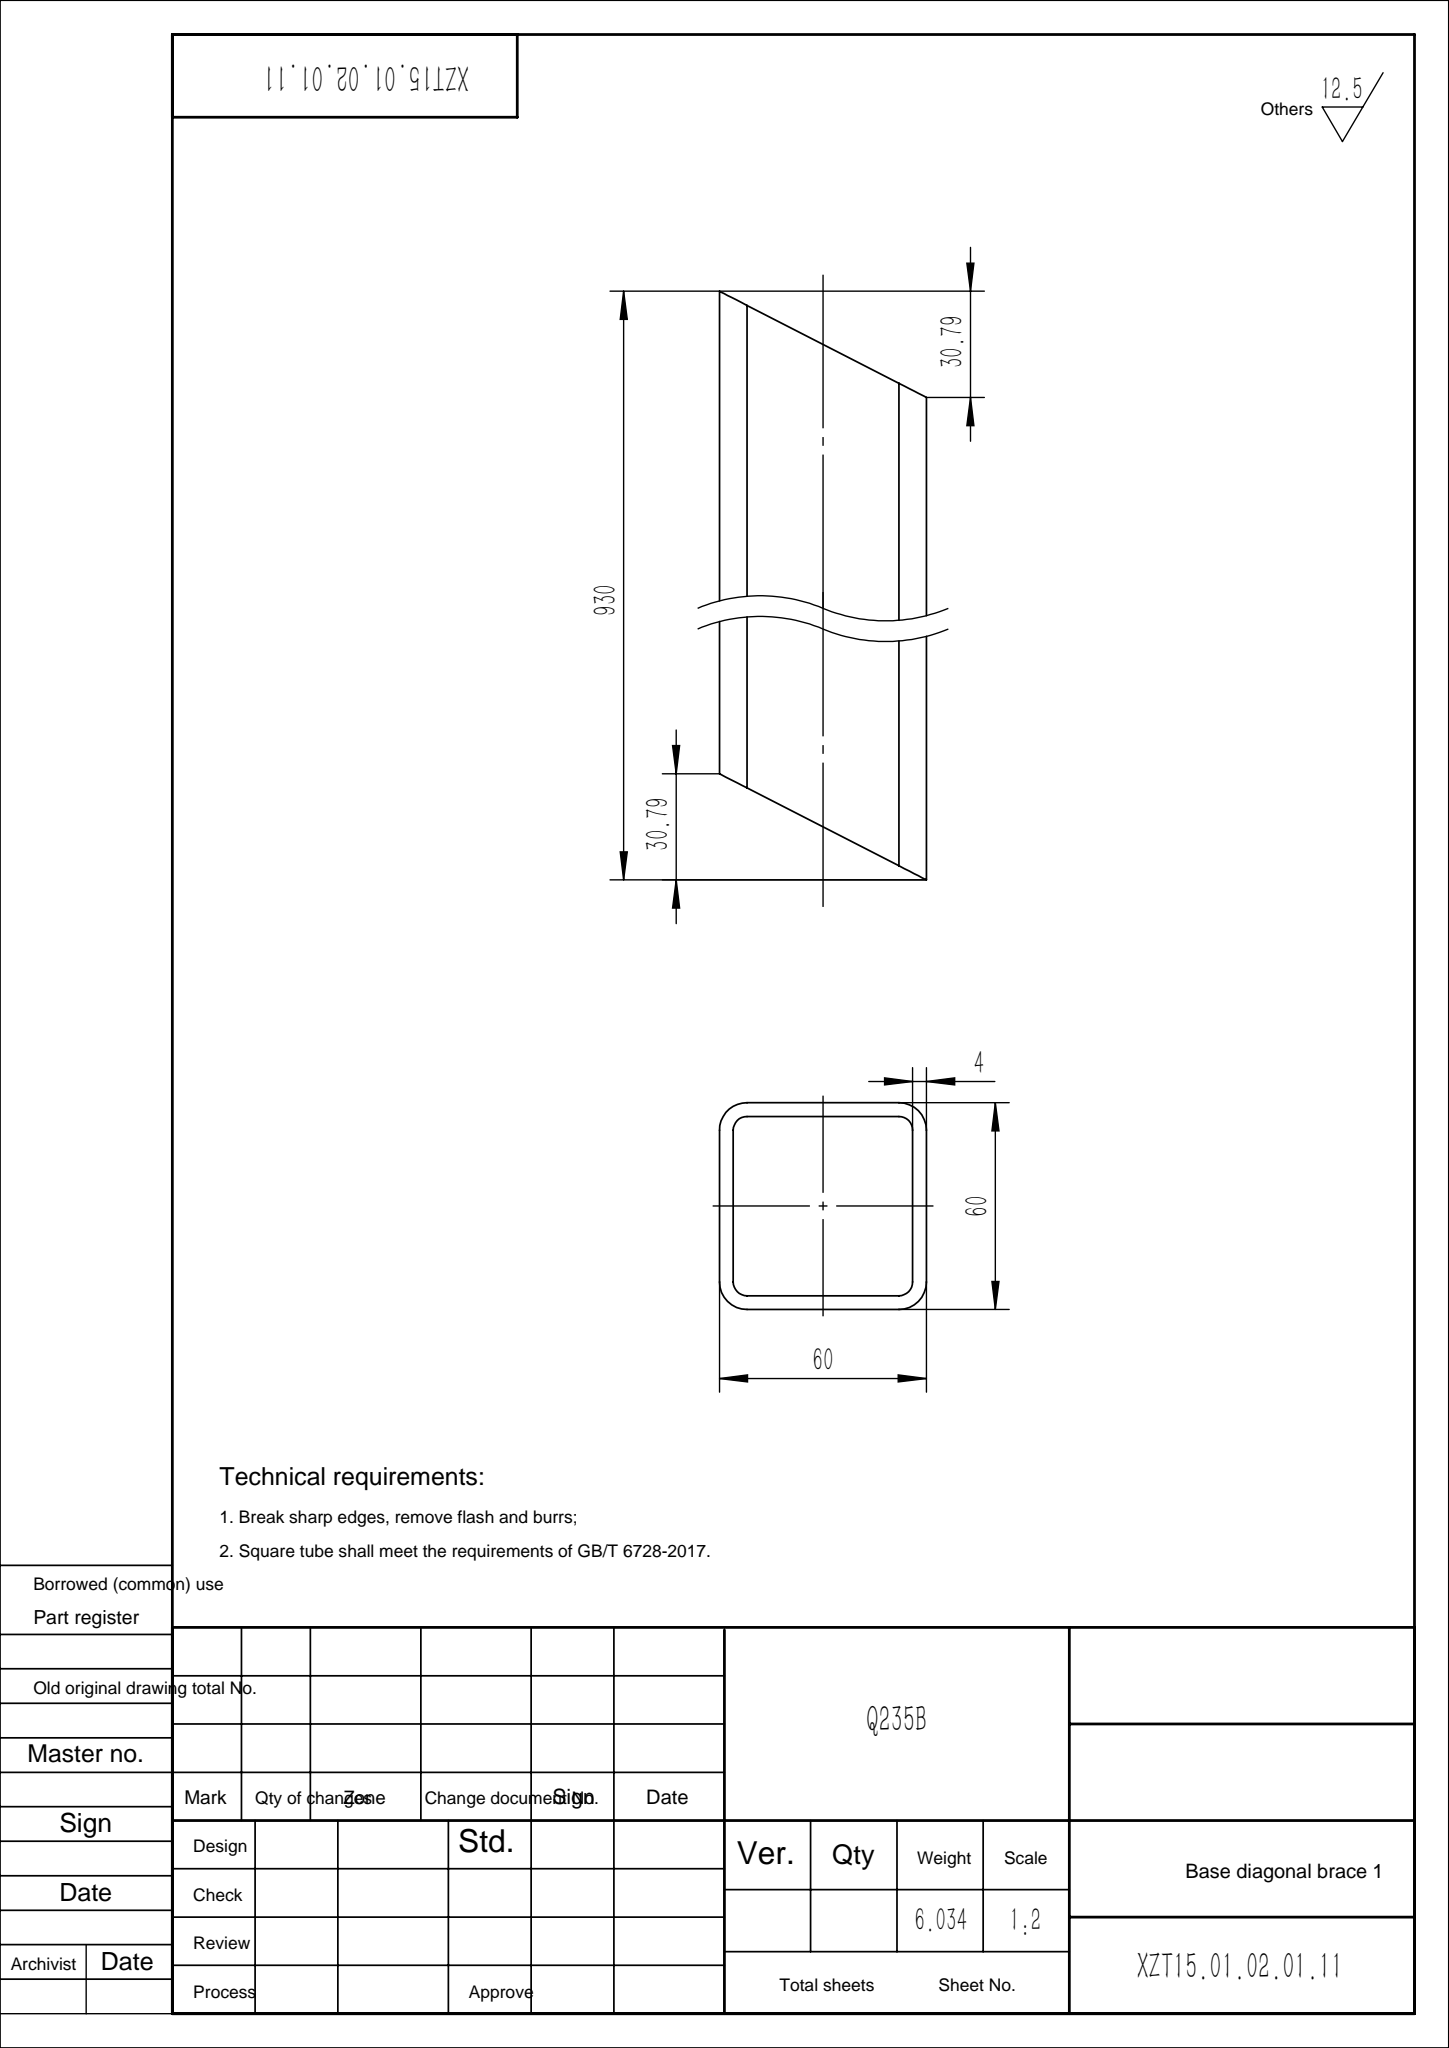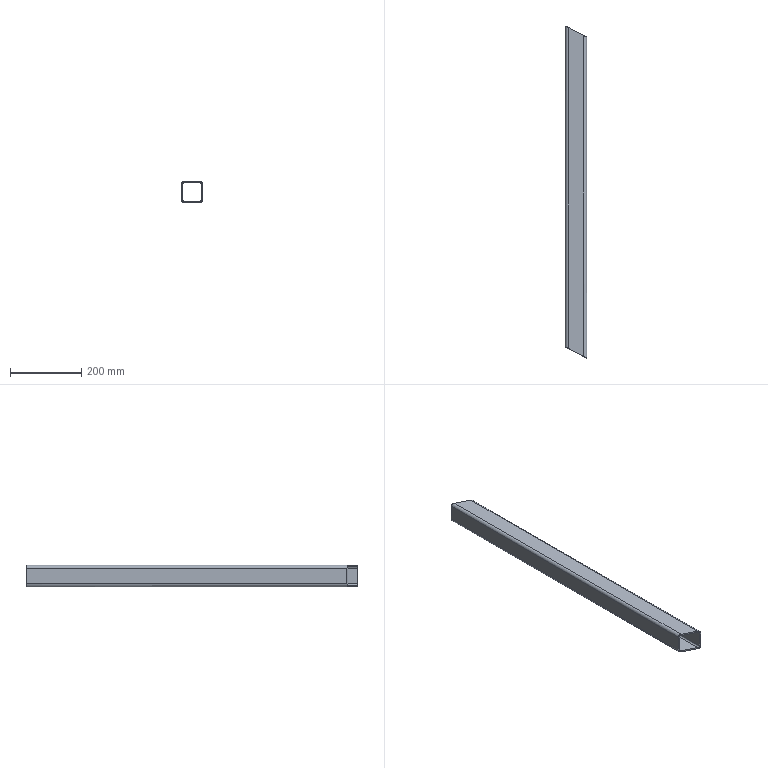Part | SolidWorks | features ICE 1, WeldMemberFeat 1, WeldmentFeature 1 | 1 solid | 18 faces | box 60 x 930 x 60 mm | volume 768639 mm3 | plane 10 | cylinder 8 | commonest cylinder face diameters 8 x4 16 x4
STEP:
#1=CARTESIAN_POINT('',(30.,899.207,-22.));
#2=VERTEX_POINT('',#1);
#3=CARTESIAN_POINT('',(30.,0.,-22.));
#4=VERTEX_POINT('',#3);
#5=CARTESIAN_POINT('',(30.,930.,-22.));
#6=DIRECTION('',(0.,-1.,0.));
#7=VECTOR('',#6,1000.);
#8=LINE('',#5,#7);
#9=EDGE_CURVE('',#2,#4,#8,.T.);
#10=ORIENTED_EDGE('',*,*,#9,.F.);
#11=CARTESIAN_POINT('',(30.,899.207,22.));
#12=VERTEX_POINT('',#11);
#13=CARTESIAN_POINT('',(30.,899.207,-30.));
#14=DIRECTION('',(0.,0.,1.));
#15=VECTOR('',#14,1000.);
#16=LINE('',#13,#15);
#17=EDGE_CURVE('',#2,#12,#16,.T.);
#18=ORIENTED_EDGE('',*,*,#17,.T.);
#19=CARTESIAN_POINT('',(30.,0.,22.));
#20=VERTEX_POINT('',#19);
#21=CARTESIAN_POINT('',(30.,930.,22.));
#22=DIRECTION('',(0.,-1.,0.));
#23=VECTOR('',#22,1000.);
#24=LINE('',#21,#23);
#25=EDGE_CURVE('',#12,#20,#24,.T.);
#26=ORIENTED_EDGE('',*,*,#25,.T.);
#27=CARTESIAN_POINT('',(30.,0.,-22.));
#28=DIRECTION('',(0.,0.,-1.));
#29=VECTOR('',#28,1000.);
#30=LINE('',#27,#29);
#31=EDGE_CURVE('',#20,#4,#30,.T.);
#32=ORIENTED_EDGE('',*,*,#31,.T.);
#33=EDGE_LOOP('',(#10,#18,#26,#32));
#34=FACE_OUTER_BOUND('',#33,.T.);
#35=CARTESIAN_POINT('',(30.,930.,-22.));
#36=DIRECTION('',(-1.,0.,0.));
#37=DIRECTION('',(0.,0.,1.));
#38=AXIS2_PLACEMENT_3D('',#35,#36,#37);
#39=PLANE('',#38);
#40=ADVANCED_FACE('',(#34),#39,.F.);
#41=CARTESIAN_POINT('',(-30.,930.,-22.));
#42=VERTEX_POINT('',#41);
#43=CARTESIAN_POINT('',(-30.,30.793,-22.));
#44=VERTEX_POINT('',#43);
#45=CARTESIAN_POINT('',(-30.,930.,-22.));
#46=DIRECTION('',(0.,-1.,0.));
#47=VECTOR('',#46,1000.);
#48=LINE('',#45,#47);
#49=EDGE_CURVE('',#42,#44,#48,.T.);
#50=ORIENTED_EDGE('',*,*,#49,.T.);
#51=CARTESIAN_POINT('',(-30.,30.793,22.));
#52=VERTEX_POINT('',#51);
#53=CARTESIAN_POINT('',(-30.,30.793,-30.));
#54=DIRECTION('',(0.,0.,1.));
#55=VECTOR('',#54,1000.);
#56=LINE('',#53,#55);
#57=EDGE_CURVE('',#44,#52,#56,.T.);
#58=ORIENTED_EDGE('',*,*,#57,.T.);
#59=CARTESIAN_POINT('',(-30.,930.,22.));
#60=VERTEX_POINT('',#59);
#61=CARTESIAN_POINT('',(-30.,930.,22.));
#62=DIRECTION('',(0.,-1.,0.));
#63=VECTOR('',#62,1000.);
#64=LINE('',#61,#63);
#65=EDGE_CURVE('',#60,#52,#64,.T.);
#66=ORIENTED_EDGE('',*,*,#65,.F.);
#67=CARTESIAN_POINT('',(-30.,930.,22.));
#68=DIRECTION('',(0.,0.,1.));
#69=VECTOR('',#68,1000.);
#70=LINE('',#67,#69);
#71=EDGE_CURVE('',#42,#60,#70,.T.);
#72=ORIENTED_EDGE('',*,*,#71,.F.);
#73=EDGE_LOOP('',(#50,#58,#66,#72));
#74=FACE_OUTER_BOUND('',#73,.T.);
#75=CARTESIAN_POINT('',(-30.,930.,22.));
#76=DIRECTION('',(1.,0.,0.));
#77=DIRECTION('',(0.,0.,-1.));
#78=AXIS2_PLACEMENT_3D('',#75,#76,#77);
#79=PLANE('',#78);
#80=ADVANCED_FACE('',(#74),#79,.F.);
#81=ORIENTED_EDGE('',*,*,#49,.F.);
#82=CARTESIAN_POINT('',(-22.,925.894,-30.));
#83=VERTEX_POINT('',#82);
#84=CARTESIAN_POINT('',(-30.,930.,-22.));
#85=CARTESIAN_POINT('',(-30.,930.,-26.686));
#86=CARTESIAN_POINT('',(-26.686,928.299,-30.));
#87=CARTESIAN_POINT('',(-22.,925.894,-30.));
#88=(BOUNDED_CURVE()B_SPLINE_CURVE(3,(#84,#85,#86,#87),.UNSPECIFIED.,.F.,.T.)B_SPLINE_CURVE_WITH_KNOTS((4,4),(3.142,4.712),.UNSPECIFIED.)CURVE()GEOMETRIC_REPRESENTATION_ITEM()RATIONAL_B_SPLINE_CURVE((1.,0.8047,0.8047,1.))REPRESENTATION_ITEM(''));
#89=EDGE_CURVE('',#42,#83,#88,.T.);
#90=ORIENTED_EDGE('',*,*,#89,.T.);
#91=CARTESIAN_POINT('',(-22.,26.687,-30.));
#92=VERTEX_POINT('',#91);
#93=CARTESIAN_POINT('',(-22.,930.,-30.));
#94=DIRECTION('',(0.,-1.,0.));
#95=VECTOR('',#94,1000.);
#96=LINE('',#93,#95);
#97=EDGE_CURVE('',#83,#92,#96,.T.);
#98=ORIENTED_EDGE('',*,*,#97,.T.);
#99=CARTESIAN_POINT('',(-22.,26.687,-30.));
#100=CARTESIAN_POINT('',(-26.686,29.093,-30.));
#101=CARTESIAN_POINT('',(-30.,30.793,-26.686));
#102=CARTESIAN_POINT('',(-30.,30.793,-22.));
#103=(BOUNDED_CURVE()B_SPLINE_CURVE(3,(#99,#100,#101,#102),.UNSPECIFIED.,.F.,.T.)B_SPLINE_CURVE_WITH_KNOTS((4,4),(1.571,3.142),.UNSPECIFIED.)CURVE()GEOMETRIC_REPRESENTATION_ITEM()RATIONAL_B_SPLINE_CURVE((1.,0.8047,0.8047,1.))REPRESENTATION_ITEM(''));
#104=EDGE_CURVE('',#92,#44,#103,.T.);
#105=ORIENTED_EDGE('',*,*,#104,.T.);
#106=EDGE_LOOP('',(#81,#90,#98,#105));
#107=FACE_OUTER_BOUND('',#106,.T.);
#108=CARTESIAN_POINT('',(-22.,930.,-22.));
#109=DIRECTION('',(0.,-1.,0.));
#110=DIRECTION('',(0.,0.,-1.));
#111=AXIS2_PLACEMENT_3D('',#108,#109,#110);
#112=CYLINDRICAL_SURFACE('',#111,8.);
#113=ADVANCED_FACE('',(#107),#112,.T.);
#114=ORIENTED_EDGE('',*,*,#97,.F.);
#115=CARTESIAN_POINT('',(22.,903.313,-30.));
#116=VERTEX_POINT('',#115);
#117=CARTESIAN_POINT('',(-30.,930.,-30.));
#118=DIRECTION('',(0.8897,-0.4566,0.));
#119=VECTOR('',#118,1000.);
#120=LINE('',#117,#119);
#121=EDGE_CURVE('',#83,#116,#120,.T.);
#122=ORIENTED_EDGE('',*,*,#121,.T.);
#123=CARTESIAN_POINT('',(22.,4.106,-30.));
#124=VERTEX_POINT('',#123);
#125=CARTESIAN_POINT('',(22.,930.,-30.));
#126=DIRECTION('',(0.,-1.,0.));
#127=VECTOR('',#126,1000.);
#128=LINE('',#125,#127);
#129=EDGE_CURVE('',#116,#124,#128,.T.);
#130=ORIENTED_EDGE('',*,*,#129,.T.);
#131=CARTESIAN_POINT('',(-30.,30.793,-30.));
#132=DIRECTION('',(-0.8897,0.4566,0.));
#133=VECTOR('',#132,1000.);
#134=LINE('',#131,#133);
#135=EDGE_CURVE('',#124,#92,#134,.T.);
#136=ORIENTED_EDGE('',*,*,#135,.T.);
#137=EDGE_LOOP('',(#114,#122,#130,#136));
#138=FACE_OUTER_BOUND('',#137,.T.);
#139=CARTESIAN_POINT('',(22.,930.,-30.));
#140=DIRECTION('',(0.,0.,1.));
#141=DIRECTION('',(1.,0.,0.));
#142=AXIS2_PLACEMENT_3D('',#139,#140,#141);
#143=PLANE('',#142);
#144=ADVANCED_FACE('',(#138),#143,.F.);
#145=ORIENTED_EDGE('',*,*,#129,.F.);
#146=CARTESIAN_POINT('',(22.,903.313,-30.));
#147=CARTESIAN_POINT('',(26.686,900.907,-30.));
#148=CARTESIAN_POINT('',(30.,899.207,-26.686));
#149=CARTESIAN_POINT('',(30.,899.207,-22.));
#150=(BOUNDED_CURVE()B_SPLINE_CURVE(3,(#146,#147,#148,#149),.UNSPECIFIED.,.F.,.F.)B_SPLINE_CURVE_WITH_KNOTS((4,4),(4.712,6.283),.UNSPECIFIED.)CURVE()GEOMETRIC_REPRESENTATION_ITEM()RATIONAL_B_SPLINE_CURVE((1.,0.8047,0.8047,1.))REPRESENTATION_ITEM(''));
#151=EDGE_CURVE('',#116,#2,#150,.T.);
#152=ORIENTED_EDGE('',*,*,#151,.T.);
#153=ORIENTED_EDGE('',*,*,#9,.T.);
#154=CARTESIAN_POINT('',(30.,0.,-22.));
#155=CARTESIAN_POINT('',(30.,0.,-26.686));
#156=CARTESIAN_POINT('',(26.686,1.701,-30.));
#157=CARTESIAN_POINT('',(22.,4.106,-30.));
#158=(BOUNDED_CURVE()B_SPLINE_CURVE(3,(#154,#155,#156,#157),.UNSPECIFIED.,.F.,.T.)B_SPLINE_CURVE_WITH_KNOTS((4,4),(0.,1.571),.UNSPECIFIED.)CURVE()GEOMETRIC_REPRESENTATION_ITEM()RATIONAL_B_SPLINE_CURVE((1.,0.8047,0.8047,1.))REPRESENTATION_ITEM(''));
#159=EDGE_CURVE('',#4,#124,#158,.T.);
#160=ORIENTED_EDGE('',*,*,#159,.T.);
#161=EDGE_LOOP('',(#145,#152,#153,#160));
#162=FACE_OUTER_BOUND('',#161,.T.);
#163=CARTESIAN_POINT('',(22.,930.,-22.));
#164=DIRECTION('',(0.,-1.,0.));
#165=DIRECTION('',(0.,0.,-1.));
#166=AXIS2_PLACEMENT_3D('',#163,#164,#165);
#167=CYLINDRICAL_SURFACE('',#166,8.);
#168=ADVANCED_FACE('',(#162),#167,.T.);
#169=ORIENTED_EDGE('',*,*,#25,.F.);
#170=CARTESIAN_POINT('',(22.,903.313,30.));
#171=VERTEX_POINT('',#170);
#172=CARTESIAN_POINT('',(30.,899.207,22.));
#173=CARTESIAN_POINT('',(30.,899.207,26.686));
#174=CARTESIAN_POINT('',(26.686,900.907,30.));
#175=CARTESIAN_POINT('',(22.,903.313,30.));
#176=(BOUNDED_CURVE()B_SPLINE_CURVE(3,(#172,#173,#174,#175),.UNSPECIFIED.,.F.,.T.)B_SPLINE_CURVE_WITH_KNOTS((4,4),(0.,1.571),.UNSPECIFIED.)CURVE()GEOMETRIC_REPRESENTATION_ITEM()RATIONAL_B_SPLINE_CURVE((1.,0.8047,0.8047,1.))REPRESENTATION_ITEM(''));
#177=EDGE_CURVE('',#12,#171,#176,.T.);
#178=ORIENTED_EDGE('',*,*,#177,.T.);
#179=CARTESIAN_POINT('',(22.,4.106,30.));
#180=VERTEX_POINT('',#179);
#181=CARTESIAN_POINT('',(22.,930.,30.));
#182=DIRECTION('',(0.,-1.,0.));
#183=VECTOR('',#182,1000.);
#184=LINE('',#181,#183);
#185=EDGE_CURVE('',#171,#180,#184,.T.);
#186=ORIENTED_EDGE('',*,*,#185,.T.);
#187=CARTESIAN_POINT('',(22.,4.106,30.));
#188=CARTESIAN_POINT('',(26.686,1.701,30.));
#189=CARTESIAN_POINT('',(30.,0.,26.686));
#190=CARTESIAN_POINT('',(30.,0.,22.));
#191=(BOUNDED_CURVE()B_SPLINE_CURVE(3,(#187,#188,#189,#190),.UNSPECIFIED.,.F.,.T.)B_SPLINE_CURVE_WITH_KNOTS((4,4),(4.712,6.283),.UNSPECIFIED.)CURVE()GEOMETRIC_REPRESENTATION_ITEM()RATIONAL_B_SPLINE_CURVE((1.,0.8047,0.8047,1.))REPRESENTATION_ITEM(''));
#192=EDGE_CURVE('',#180,#20,#191,.T.);
#193=ORIENTED_EDGE('',*,*,#192,.T.);
#194=EDGE_LOOP('',(#169,#178,#186,#193));
#195=FACE_OUTER_BOUND('',#194,.T.);
#196=CARTESIAN_POINT('',(22.,930.,22.));
#197=DIRECTION('',(0.,-1.,0.));
#198=DIRECTION('',(0.,0.,-1.));
#199=AXIS2_PLACEMENT_3D('',#196,#197,#198);
#200=CYLINDRICAL_SURFACE('',#199,8.);
#201=ADVANCED_FACE('',(#195),#200,.T.);
#202=ORIENTED_EDGE('',*,*,#185,.F.);
#203=CARTESIAN_POINT('',(-22.,925.894,30.));
#204=VERTEX_POINT('',#203);
#205=CARTESIAN_POINT('',(-23.668,926.75,30.));
#206=DIRECTION('',(-0.8897,0.4566,0.));
#207=VECTOR('',#206,1000.);
#208=LINE('',#205,#207);
#209=EDGE_CURVE('',#171,#204,#208,.T.);
#210=ORIENTED_EDGE('',*,*,#209,.T.);
#211=CARTESIAN_POINT('',(-22.,26.687,30.));
#212=VERTEX_POINT('',#211);
#213=CARTESIAN_POINT('',(-22.,930.,30.));
#214=DIRECTION('',(0.,-1.,0.));
#215=VECTOR('',#214,1000.);
#216=LINE('',#213,#215);
#217=EDGE_CURVE('',#204,#212,#216,.T.);
#218=ORIENTED_EDGE('',*,*,#217,.T.);
#219=CARTESIAN_POINT('',(-388.946,215.012,30.));
#220=DIRECTION('',(0.8897,-0.4566,0.));
#221=VECTOR('',#220,1000.);
#222=LINE('',#219,#221);
#223=EDGE_CURVE('',#212,#180,#222,.T.);
#224=ORIENTED_EDGE('',*,*,#223,.T.);
#225=EDGE_LOOP('',(#202,#210,#218,#224));
#226=FACE_OUTER_BOUND('',#225,.T.);
#227=CARTESIAN_POINT('',(-22.,930.,30.));
#228=DIRECTION('',(0.,0.,-1.));
#229=DIRECTION('',(-1.,0.,0.));
#230=AXIS2_PLACEMENT_3D('',#227,#228,#229);
#231=PLANE('',#230);
#232=ADVANCED_FACE('',(#226),#231,.F.);
#233=ORIENTED_EDGE('',*,*,#217,.F.);
#234=CARTESIAN_POINT('',(-22.,925.894,30.));
#235=CARTESIAN_POINT('',(-26.686,928.299,30.));
#236=CARTESIAN_POINT('',(-30.,930.,26.686));
#237=CARTESIAN_POINT('',(-30.,930.,22.));
#238=(BOUNDED_CURVE()B_SPLINE_CURVE(3,(#234,#235,#236,#237),.UNSPECIFIED.,.F.,.T.)B_SPLINE_CURVE_WITH_KNOTS((4,4),(1.571,3.142),.UNSPECIFIED.)CURVE()GEOMETRIC_REPRESENTATION_ITEM()RATIONAL_B_SPLINE_CURVE((1.,0.8047,0.8047,1.))REPRESENTATION_ITEM(''));
#239=EDGE_CURVE('',#204,#60,#238,.T.);
#240=ORIENTED_EDGE('',*,*,#239,.T.);
#241=ORIENTED_EDGE('',*,*,#65,.T.);
#242=CARTESIAN_POINT('',(-30.,30.793,22.));
#243=CARTESIAN_POINT('',(-30.,30.793,26.686));
#244=CARTESIAN_POINT('',(-26.686,29.093,30.));
#245=CARTESIAN_POINT('',(-22.,26.687,30.));
#246=(BOUNDED_CURVE()B_SPLINE_CURVE(3,(#242,#243,#244,#245),.UNSPECIFIED.,.F.,.F.)B_SPLINE_CURVE_WITH_KNOTS((4,4),(3.142,4.712),.UNSPECIFIED.)CURVE()GEOMETRIC_REPRESENTATION_ITEM()RATIONAL_B_SPLINE_CURVE((1.,0.8047,0.8047,1.))REPRESENTATION_ITEM(''));
#247=EDGE_CURVE('',#52,#212,#246,.T.);
#248=ORIENTED_EDGE('',*,*,#247,.T.);
#249=EDGE_LOOP('',(#233,#240,#241,#248));
#250=FACE_OUTER_BOUND('',#249,.T.);
#251=CARTESIAN_POINT('',(-22.,930.,22.));
#252=DIRECTION('',(0.,-1.,0.));
#253=DIRECTION('',(0.,0.,-1.));
#254=AXIS2_PLACEMENT_3D('',#251,#252,#253);
#255=CYLINDRICAL_SURFACE('',#254,8.);
#256=ADVANCED_FACE('',(#250),#255,.T.);
#257=CARTESIAN_POINT('',(22.,4.106,26.));
#258=VERTEX_POINT('',#257);
#259=CARTESIAN_POINT('',(26.,2.053,22.));
#260=VERTEX_POINT('',#259);
#261=CARTESIAN_POINT('',(22.,4.106,26.));
#262=CARTESIAN_POINT('',(24.343,2.903,26.));
#263=CARTESIAN_POINT('',(26.,2.053,24.343));
#264=CARTESIAN_POINT('',(26.,2.053,22.));
#265=(BOUNDED_CURVE()B_SPLINE_CURVE(3,(#261,#262,#263,#264),.UNSPECIFIED.,.F.,.T.)B_SPLINE_CURVE_WITH_KNOTS((4,4),(4.712,6.283),.UNSPECIFIED.)CURVE()GEOMETRIC_REPRESENTATION_ITEM()RATIONAL_B_SPLINE_CURVE((1.,0.8047,0.8047,1.))REPRESENTATION_ITEM(''));
#266=EDGE_CURVE('',#258,#260,#265,.T.);
#267=ORIENTED_EDGE('',*,*,#266,.T.);
#268=CARTESIAN_POINT('',(26.,2.053,-22.));
#269=VERTEX_POINT('',#268);
#270=CARTESIAN_POINT('',(26.,2.053,-22.));
#271=DIRECTION('',(0.,0.,-1.));
#272=VECTOR('',#271,1000.);
#273=LINE('',#270,#272);
#274=EDGE_CURVE('',#260,#269,#273,.T.);
#275=ORIENTED_EDGE('',*,*,#274,.T.);
#276=CARTESIAN_POINT('',(22.,4.106,-26.));
#277=VERTEX_POINT('',#276);
#278=CARTESIAN_POINT('',(26.,2.053,-22.));
#279=CARTESIAN_POINT('',(26.,2.053,-24.343));
#280=CARTESIAN_POINT('',(24.343,2.903,-26.));
#281=CARTESIAN_POINT('',(22.,4.106,-26.));
#282=(BOUNDED_CURVE()B_SPLINE_CURVE(3,(#278,#279,#280,#281),.UNSPECIFIED.,.F.,.T.)B_SPLINE_CURVE_WITH_KNOTS((4,4),(0.,1.571),.UNSPECIFIED.)CURVE()GEOMETRIC_REPRESENTATION_ITEM()RATIONAL_B_SPLINE_CURVE((1.,0.8047,0.8047,1.))REPRESENTATION_ITEM(''));
#283=EDGE_CURVE('',#269,#277,#282,.T.);
#284=ORIENTED_EDGE('',*,*,#283,.T.);
#285=CARTESIAN_POINT('',(-22.,26.687,-26.));
#286=VERTEX_POINT('',#285);
#287=CARTESIAN_POINT('',(-354.12,197.138,-26.));
#288=DIRECTION('',(-0.8897,0.4566,0.));
#289=VECTOR('',#288,1000.);
#290=LINE('',#287,#289);
#291=EDGE_CURVE('',#277,#286,#290,.T.);
#292=ORIENTED_EDGE('',*,*,#291,.T.);
#293=CARTESIAN_POINT('',(-26.,28.74,-22.));
#294=VERTEX_POINT('',#293);
#295=CARTESIAN_POINT('',(-22.,26.687,-26.));
#296=CARTESIAN_POINT('',(-24.343,27.89,-26.));
#297=CARTESIAN_POINT('',(-26.,28.74,-24.343));
#298=CARTESIAN_POINT('',(-26.,28.74,-22.));
#299=(BOUNDED_CURVE()B_SPLINE_CURVE(3,(#295,#296,#297,#298),.UNSPECIFIED.,.F.,.T.)B_SPLINE_CURVE_WITH_KNOTS((4,4),(1.571,3.142),.UNSPECIFIED.)CURVE()GEOMETRIC_REPRESENTATION_ITEM()RATIONAL_B_SPLINE_CURVE((1.,0.8047,0.8047,1.))REPRESENTATION_ITEM(''));
#300=EDGE_CURVE('',#286,#294,#299,.T.);
#301=ORIENTED_EDGE('',*,*,#300,.T.);
#302=CARTESIAN_POINT('',(-26.,28.74,22.));
#303=VERTEX_POINT('',#302);
#304=CARTESIAN_POINT('',(-26.,28.74,22.));
#305=DIRECTION('',(0.,0.,1.));
#306=VECTOR('',#305,1000.);
#307=LINE('',#304,#306);
#308=EDGE_CURVE('',#294,#303,#307,.T.);
#309=ORIENTED_EDGE('',*,*,#308,.T.);
#310=CARTESIAN_POINT('',(-22.,26.687,26.));
#311=VERTEX_POINT('',#310);
#312=CARTESIAN_POINT('',(-26.,28.74,22.));
#313=CARTESIAN_POINT('',(-26.,28.74,24.343));
#314=CARTESIAN_POINT('',(-24.343,27.89,26.));
#315=CARTESIAN_POINT('',(-22.,26.687,26.));
#316=(BOUNDED_CURVE()B_SPLINE_CURVE(3,(#312,#313,#314,#315),.UNSPECIFIED.,.F.,.F.)B_SPLINE_CURVE_WITH_KNOTS((4,4),(3.142,4.712),.UNSPECIFIED.)CURVE()GEOMETRIC_REPRESENTATION_ITEM()RATIONAL_B_SPLINE_CURVE((1.,0.8047,0.8047,1.))REPRESENTATION_ITEM(''));
#317=EDGE_CURVE('',#303,#311,#316,.T.);
#318=ORIENTED_EDGE('',*,*,#317,.T.);
#319=CARTESIAN_POINT('',(-388.946,215.012,26.));
#320=DIRECTION('',(0.8897,-0.4566,0.));
#321=VECTOR('',#320,1000.);
#322=LINE('',#319,#321);
#323=EDGE_CURVE('',#311,#258,#322,.T.);
#324=ORIENTED_EDGE('',*,*,#323,.T.);
#325=EDGE_LOOP('',(#267,#275,#284,#292,#301,#309,#318,#324));
#326=FACE_BOUND('',#325,.T.);
#327=ORIENTED_EDGE('',*,*,#57,.F.);
#328=ORIENTED_EDGE('',*,*,#104,.F.);
#329=ORIENTED_EDGE('',*,*,#135,.F.);
#330=ORIENTED_EDGE('',*,*,#159,.F.);
#331=ORIENTED_EDGE('',*,*,#31,.F.);
#332=ORIENTED_EDGE('',*,*,#192,.F.);
#333=ORIENTED_EDGE('',*,*,#223,.F.);
#334=ORIENTED_EDGE('',*,*,#247,.F.);
#335=EDGE_LOOP('',(#327,#328,#329,#330,#331,#332,#333,#334));
#336=FACE_OUTER_BOUND('',#335,.T.);
#337=CARTESIAN_POINT('',(-30.,30.793,-30.));
#338=DIRECTION('',(0.4566,0.8897,0.));
#339=DIRECTION('',(-0.8897,0.4566,0.));
#340=AXIS2_PLACEMENT_3D('',#337,#338,#339);
#341=PLANE('',#340);
#342=ADVANCED_FACE('',(#326,#336),#341,.F.);
#343=CARTESIAN_POINT('',(26.,901.26,22.));
#344=VERTEX_POINT('',#343);
#345=CARTESIAN_POINT('',(22.,903.313,26.));
#346=VERTEX_POINT('',#345);
#347=CARTESIAN_POINT('',(26.,901.26,22.));
#348=CARTESIAN_POINT('',(26.,901.26,24.343));
#349=CARTESIAN_POINT('',(24.343,902.11,26.));
#350=CARTESIAN_POINT('',(22.,903.313,26.));
#351=(BOUNDED_CURVE()B_SPLINE_CURVE(3,(#347,#348,#349,#350),.UNSPECIFIED.,.F.,.T.)B_SPLINE_CURVE_WITH_KNOTS((4,4),(0.,1.571),.UNSPECIFIED.)CURVE()GEOMETRIC_REPRESENTATION_ITEM()RATIONAL_B_SPLINE_CURVE((1.,0.8047,0.8047,1.))REPRESENTATION_ITEM(''));
#352=EDGE_CURVE('',#344,#346,#351,.T.);
#353=ORIENTED_EDGE('',*,*,#352,.T.);
#354=CARTESIAN_POINT('',(-22.,925.894,26.));
#355=VERTEX_POINT('',#354);
#356=CARTESIAN_POINT('',(-23.668,926.75,26.));
#357=DIRECTION('',(-0.8897,0.4566,0.));
#358=VECTOR('',#357,1000.);
#359=LINE('',#356,#358);
#360=EDGE_CURVE('',#346,#355,#359,.T.);
#361=ORIENTED_EDGE('',*,*,#360,.T.);
#362=CARTESIAN_POINT('',(-26.,927.947,22.));
#363=VERTEX_POINT('',#362);
#364=CARTESIAN_POINT('',(-22.,925.894,26.));
#365=CARTESIAN_POINT('',(-24.343,927.097,26.));
#366=CARTESIAN_POINT('',(-26.,927.947,24.343));
#367=CARTESIAN_POINT('',(-26.,927.947,22.));
#368=(BOUNDED_CURVE()B_SPLINE_CURVE(3,(#364,#365,#366,#367),.UNSPECIFIED.,.F.,.F.)B_SPLINE_CURVE_WITH_KNOTS((4,4),(1.571,3.142),.UNSPECIFIED.)CURVE()GEOMETRIC_REPRESENTATION_ITEM()RATIONAL_B_SPLINE_CURVE((1.,0.8047,0.8047,1.))REPRESENTATION_ITEM(''));
#369=EDGE_CURVE('',#355,#363,#368,.T.);
#370=ORIENTED_EDGE('',*,*,#369,.T.);
#371=CARTESIAN_POINT('',(-26.,927.947,-22.));
#372=VERTEX_POINT('',#371);
#373=CARTESIAN_POINT('',(-26.,927.947,22.));
#374=DIRECTION('',(0.,0.,-1.));
#375=VECTOR('',#374,1000.);
#376=LINE('',#373,#375);
#377=EDGE_CURVE('',#363,#372,#376,.T.);
#378=ORIENTED_EDGE('',*,*,#377,.T.);
#379=CARTESIAN_POINT('',(-22.,925.894,-26.));
#380=VERTEX_POINT('',#379);
#381=CARTESIAN_POINT('',(-26.,927.947,-22.));
#382=CARTESIAN_POINT('',(-26.,927.947,-24.343));
#383=CARTESIAN_POINT('',(-24.343,927.097,-26.));
#384=CARTESIAN_POINT('',(-22.,925.894,-26.));
#385=(BOUNDED_CURVE()B_SPLINE_CURVE(3,(#381,#382,#383,#384),.UNSPECIFIED.,.F.,.T.)B_SPLINE_CURVE_WITH_KNOTS((4,4),(3.142,4.712),.UNSPECIFIED.)CURVE()GEOMETRIC_REPRESENTATION_ITEM()RATIONAL_B_SPLINE_CURVE((1.,0.8047,0.8047,1.))REPRESENTATION_ITEM(''));
#386=EDGE_CURVE('',#372,#380,#385,.T.);
#387=ORIENTED_EDGE('',*,*,#386,.T.);
#388=CARTESIAN_POINT('',(22.,903.313,-26.));
#389=VERTEX_POINT('',#388);
#390=CARTESIAN_POINT('',(11.159,908.876,-26.));
#391=DIRECTION('',(0.8897,-0.4566,0.));
#392=VECTOR('',#391,1000.);
#393=LINE('',#390,#392);
#394=EDGE_CURVE('',#380,#389,#393,.T.);
#395=ORIENTED_EDGE('',*,*,#394,.T.);
#396=CARTESIAN_POINT('',(26.,901.26,-22.));
#397=VERTEX_POINT('',#396);
#398=CARTESIAN_POINT('',(22.,903.313,-26.));
#399=CARTESIAN_POINT('',(24.343,902.11,-26.));
#400=CARTESIAN_POINT('',(26.,901.26,-24.343));
#401=CARTESIAN_POINT('',(26.,901.26,-22.));
#402=(BOUNDED_CURVE()B_SPLINE_CURVE(3,(#398,#399,#400,#401),.UNSPECIFIED.,.F.,.T.)B_SPLINE_CURVE_WITH_KNOTS((4,4),(4.712,6.283),.UNSPECIFIED.)CURVE()GEOMETRIC_REPRESENTATION_ITEM()RATIONAL_B_SPLINE_CURVE((1.,0.8047,0.8047,1.))REPRESENTATION_ITEM(''));
#403=EDGE_CURVE('',#389,#397,#402,.T.);
#404=ORIENTED_EDGE('',*,*,#403,.T.);
#405=CARTESIAN_POINT('',(26.,901.26,-22.));
#406=DIRECTION('',(0.,0.,1.));
#407=VECTOR('',#406,1000.);
#408=LINE('',#405,#407);
#409=EDGE_CURVE('',#397,#344,#408,.T.);
#410=ORIENTED_EDGE('',*,*,#409,.T.);
#411=EDGE_LOOP('',(#353,#361,#370,#378,#387,#395,#404,#410));
#412=FACE_BOUND('',#411,.T.);
#413=ORIENTED_EDGE('',*,*,#209,.F.);
#414=ORIENTED_EDGE('',*,*,#177,.F.);
#415=ORIENTED_EDGE('',*,*,#17,.F.);
#416=ORIENTED_EDGE('',*,*,#151,.F.);
#417=ORIENTED_EDGE('',*,*,#121,.F.);
#418=ORIENTED_EDGE('',*,*,#89,.F.);
#419=ORIENTED_EDGE('',*,*,#71,.T.);
#420=ORIENTED_EDGE('',*,*,#239,.F.);
#421=EDGE_LOOP('',(#413,#414,#415,#416,#417,#418,#419,#420));
#422=FACE_OUTER_BOUND('',#421,.T.);
#423=CARTESIAN_POINT('',(-30.,930.,-30.));
#424=DIRECTION('',(-0.4566,-0.8897,0.));
#425=DIRECTION('',(0.8897,-0.4566,0.));
#426=AXIS2_PLACEMENT_3D('',#423,#424,#425);
#427=PLANE('',#426);
#428=ADVANCED_FACE('',(#412,#422),#427,.F.);
#429=ORIENTED_EDGE('',*,*,#352,.F.);
#430=CARTESIAN_POINT('',(26.,930.,22.));
#431=DIRECTION('',(0.,-1.,0.));
#432=VECTOR('',#431,1000.);
#433=LINE('',#430,#432);
#434=EDGE_CURVE('',#344,#260,#433,.T.);
#435=ORIENTED_EDGE('',*,*,#434,.T.);
#436=ORIENTED_EDGE('',*,*,#266,.F.);
#437=CARTESIAN_POINT('',(22.,930.,26.));
#438=DIRECTION('',(0.,-1.,0.));
#439=VECTOR('',#438,1000.);
#440=LINE('',#437,#439);
#441=EDGE_CURVE('',#346,#258,#440,.T.);
#442=ORIENTED_EDGE('',*,*,#441,.F.);
#443=EDGE_LOOP('',(#429,#435,#436,#442));
#444=FACE_OUTER_BOUND('',#443,.T.);
#445=CARTESIAN_POINT('',(22.,930.,22.));
#446=DIRECTION('',(0.,-1.,0.));
#447=DIRECTION('',(0.,0.,-1.));
#448=AXIS2_PLACEMENT_3D('',#445,#446,#447);
#449=CYLINDRICAL_SURFACE('',#448,4.);
#450=ADVANCED_FACE('',(#444),#449,.F.);
#451=ORIENTED_EDGE('',*,*,#360,.F.);
#452=ORIENTED_EDGE('',*,*,#441,.T.);
#453=ORIENTED_EDGE('',*,*,#323,.F.);
#454=CARTESIAN_POINT('',(-22.,930.,26.));
#455=DIRECTION('',(0.,-1.,0.));
#456=VECTOR('',#455,1000.);
#457=LINE('',#454,#456);
#458=EDGE_CURVE('',#355,#311,#457,.T.);
#459=ORIENTED_EDGE('',*,*,#458,.F.);
#460=EDGE_LOOP('',(#451,#452,#453,#459));
#461=FACE_OUTER_BOUND('',#460,.T.);
#462=CARTESIAN_POINT('',(-22.,930.,26.));
#463=DIRECTION('',(0.,0.,-1.));
#464=DIRECTION('',(-1.,0.,0.));
#465=AXIS2_PLACEMENT_3D('',#462,#463,#464);
#466=PLANE('',#465);
#467=ADVANCED_FACE('',(#461),#466,.T.);
#468=ORIENTED_EDGE('',*,*,#369,.F.);
#469=ORIENTED_EDGE('',*,*,#458,.T.);
#470=ORIENTED_EDGE('',*,*,#317,.F.);
#471=CARTESIAN_POINT('',(-26.,930.,22.));
#472=DIRECTION('',(0.,-1.,0.));
#473=VECTOR('',#472,1000.);
#474=LINE('',#471,#473);
#475=EDGE_CURVE('',#363,#303,#474,.T.);
#476=ORIENTED_EDGE('',*,*,#475,.F.);
#477=EDGE_LOOP('',(#468,#469,#470,#476));
#478=FACE_OUTER_BOUND('',#477,.T.);
#479=CARTESIAN_POINT('',(-22.,930.,22.));
#480=DIRECTION('',(0.,-1.,0.));
#481=DIRECTION('',(0.,0.,-1.));
#482=AXIS2_PLACEMENT_3D('',#479,#480,#481);
#483=CYLINDRICAL_SURFACE('',#482,4.);
#484=ADVANCED_FACE('',(#478),#483,.F.);
#485=ORIENTED_EDGE('',*,*,#377,.F.);
#486=ORIENTED_EDGE('',*,*,#475,.T.);
#487=ORIENTED_EDGE('',*,*,#308,.F.);
#488=CARTESIAN_POINT('',(-26.,930.,-22.));
#489=DIRECTION('',(0.,-1.,0.));
#490=VECTOR('',#489,1000.);
#491=LINE('',#488,#490);
#492=EDGE_CURVE('',#372,#294,#491,.T.);
#493=ORIENTED_EDGE('',*,*,#492,.F.);
#494=EDGE_LOOP('',(#485,#486,#487,#493));
#495=FACE_OUTER_BOUND('',#494,.T.);
#496=CARTESIAN_POINT('',(-26.,930.,22.));
#497=DIRECTION('',(1.,0.,0.));
#498=DIRECTION('',(0.,0.,-1.));
#499=AXIS2_PLACEMENT_3D('',#496,#497,#498);
#500=PLANE('',#499);
#501=ADVANCED_FACE('',(#495),#500,.T.);
#502=ORIENTED_EDGE('',*,*,#386,.F.);
#503=ORIENTED_EDGE('',*,*,#492,.T.);
#504=ORIENTED_EDGE('',*,*,#300,.F.);
#505=CARTESIAN_POINT('',(-22.,930.,-26.));
#506=DIRECTION('',(0.,-1.,0.));
#507=VECTOR('',#506,1000.);
#508=LINE('',#505,#507);
#509=EDGE_CURVE('',#380,#286,#508,.T.);
#510=ORIENTED_EDGE('',*,*,#509,.F.);
#511=EDGE_LOOP('',(#502,#503,#504,#510));
#512=FACE_OUTER_BOUND('',#511,.T.);
#513=CARTESIAN_POINT('',(-22.,930.,-22.));
#514=DIRECTION('',(0.,-1.,0.));
#515=DIRECTION('',(0.,0.,-1.));
#516=AXIS2_PLACEMENT_3D('',#513,#514,#515);
#517=CYLINDRICAL_SURFACE('',#516,4.);
#518=ADVANCED_FACE('',(#512),#517,.F.);
#519=ORIENTED_EDGE('',*,*,#394,.F.);
#520=ORIENTED_EDGE('',*,*,#509,.T.);
#521=ORIENTED_EDGE('',*,*,#291,.F.);
#522=CARTESIAN_POINT('',(22.,930.,-26.));
#523=DIRECTION('',(0.,-1.,0.));
#524=VECTOR('',#523,1000.);
#525=LINE('',#522,#524);
#526=EDGE_CURVE('',#389,#277,#525,.T.);
#527=ORIENTED_EDGE('',*,*,#526,.F.);
#528=EDGE_LOOP('',(#519,#520,#521,#527));
#529=FACE_OUTER_BOUND('',#528,.T.);
#530=CARTESIAN_POINT('',(22.,930.,-26.));
#531=DIRECTION('',(0.,0.,1.));
#532=DIRECTION('',(1.,0.,0.));
#533=AXIS2_PLACEMENT_3D('',#530,#531,#532);
#534=PLANE('',#533);
#535=ADVANCED_FACE('',(#529),#534,.T.);
#536=ORIENTED_EDGE('',*,*,#403,.F.);
#537=ORIENTED_EDGE('',*,*,#526,.T.);
#538=ORIENTED_EDGE('',*,*,#283,.F.);
#539=CARTESIAN_POINT('',(26.,930.,-22.));
#540=DIRECTION('',(0.,-1.,0.));
#541=VECTOR('',#540,1000.);
#542=LINE('',#539,#541);
#543=EDGE_CURVE('',#397,#269,#542,.T.);
#544=ORIENTED_EDGE('',*,*,#543,.F.);
#545=EDGE_LOOP('',(#536,#537,#538,#544));
#546=FACE_OUTER_BOUND('',#545,.T.);
#547=CARTESIAN_POINT('',(22.,930.,-22.));
#548=DIRECTION('',(0.,-1.,0.));
#549=DIRECTION('',(0.,0.,-1.));
#550=AXIS2_PLACEMENT_3D('',#547,#548,#549);
#551=CYLINDRICAL_SURFACE('',#550,4.);
#552=ADVANCED_FACE('',(#546),#551,.F.);
#553=ORIENTED_EDGE('',*,*,#409,.F.);
#554=ORIENTED_EDGE('',*,*,#543,.T.);
#555=ORIENTED_EDGE('',*,*,#274,.F.);
#556=ORIENTED_EDGE('',*,*,#434,.F.);
#557=EDGE_LOOP('',(#553,#554,#555,#556));
#558=FACE_OUTER_BOUND('',#557,.T.);
#559=CARTESIAN_POINT('',(26.,930.,-22.));
#560=DIRECTION('',(-1.,0.,0.));
#561=DIRECTION('',(0.,0.,1.));
#562=AXIS2_PLACEMENT_3D('',#559,#560,#561);
#563=PLANE('',#562);
#564=ADVANCED_FACE('',(#558),#563,.T.);
#565=CLOSED_SHELL('',(#40,#80,#113,#144,#168,#201,#232,#256,#342,#428,#450,#467,#484,#501,#518,#535,#552,#564));
#566=MANIFOLD_SOLID_BREP('',#565);
#567=CARTESIAN_POINT('',(0.,0.,0.));
#568=DIRECTION('',(0.,0.,1.));
#569=DIRECTION('',(1.,0.,0.));
#570=AXIS2_PLACEMENT_3D('',#567,#568,#569);
#571=(LENGTH_UNIT()NAMED_UNIT(*)SI_UNIT(.MILLI.,.METRE.));
#572=UNCERTAINTY_MEASURE_WITH_UNIT(LENGTH_MEASURE(0.00001),#571,'','');
#573=(NAMED_UNIT(*)PLANE_ANGLE_UNIT()SI_UNIT($,.RADIAN.));
#574=(NAMED_UNIT(*)SI_UNIT($,.STERADIAN.)SOLID_ANGLE_UNIT());
#575=(GEOMETRIC_REPRESENTATION_CONTEXT(3)GLOBAL_UNCERTAINTY_ASSIGNED_CONTEXT((#572))GLOBAL_UNIT_ASSIGNED_CONTEXT((#571,#573,#574))REPRESENTATION_CONTEXT('',''));
#576=ADVANCED_BREP_SHAPE_REPRESENTATION('',(#566,#570),#575);